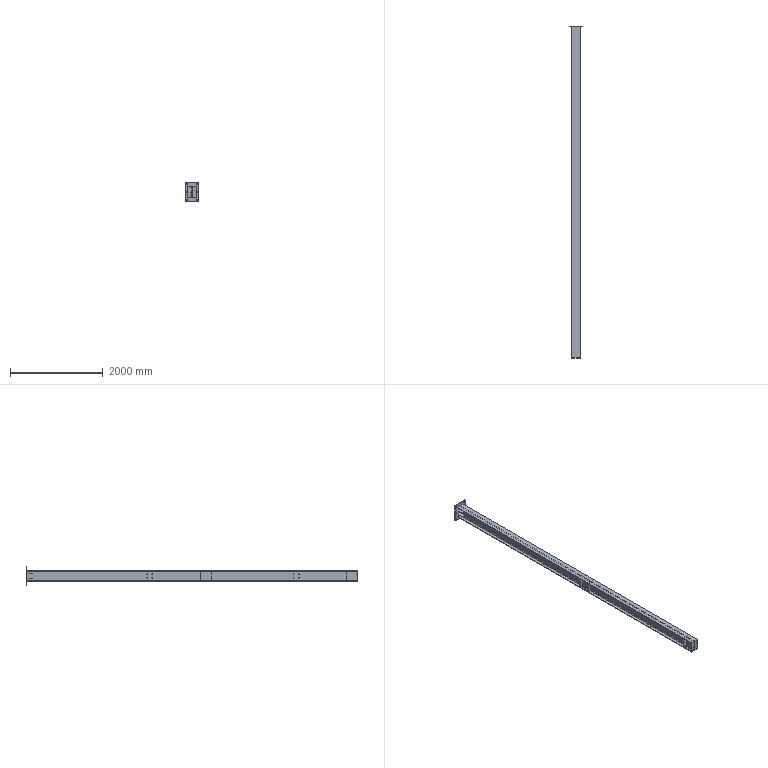Part | STEP file | PN_0027 steel column HM250X175=7134_Default<As Machined> | 14 solids | 165 faces | box 300 x 7150 x 400 mm | volume 42980324 mm3 | plane 113 | cylinder 47 | spline 4 | cone 1 | commonest cylinder face diameters 18 x16 21.5 x12 26 x10 6.8 x5 20 x4